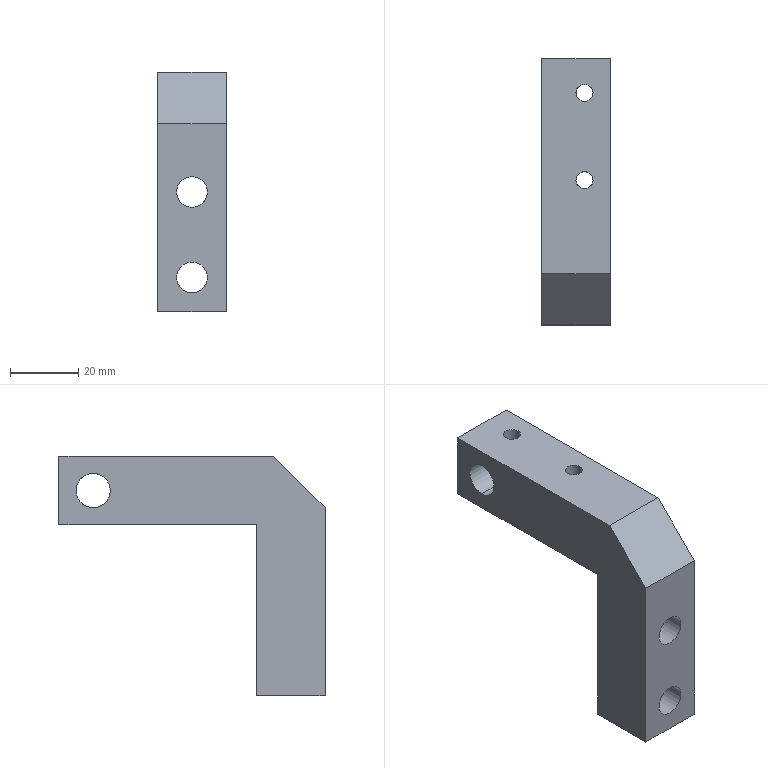Part | STEP file | Positioning_id2270_x_t | 1 solid | 32 faces | box 20 x 77.797 x 69.995 mm | volume 41126 mm3 | cylinder 20 | plane 12 | commonest cylinder face diameters 5 x8 9 x4 10 x4 14 x4